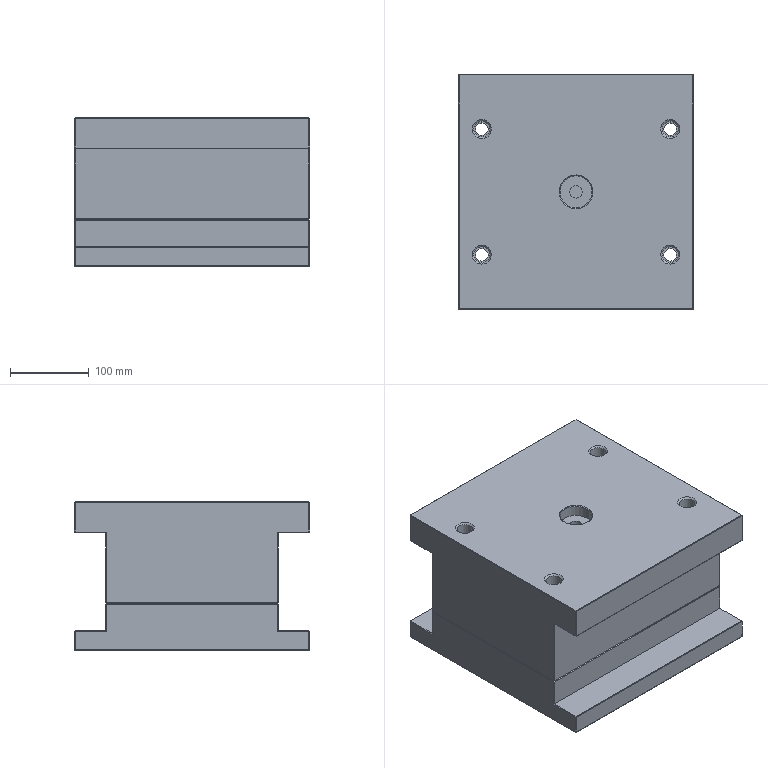NC program | NX | posted with a generic post | part box 300 x 300 x 190 mm
Lines 9219 to 10052 of 34829:
(CAVITY_MILL_COPY_COPY_COPY , TOOL : D6)
N18436 T06 M6
N18438 G17 G43 G0 G90 X-0.783 Y1.63 Z30. S2500 H6 M3
N18440 Z-58.5
N18442 G94 G1 X-1.101 Y1.448 Z-58.519 F1000.
N18444 X-1.436 Y1.116 Z-58.544
N18446 X-1.637 Y0.793 Z-58.564
N18448 X-1.795 Y0.295 Z-58.591
N18450 X-1.805 Y-0.227 Z-58.619
N18452 X-1.666 Y-0.731 Z-58.646
N18454 X-1.389 Y-1.174 Z-58.673
N18456 X-0.999 Y-1.52 Z-58.701
N18458 X-0.526 Y-1.741 Z-58.728
N18460 X-0.151 Y-1.813 Z-58.748
N18462 X0.002 Y-1.819 Z-58.756
N18464 X0.38 Y-1.779 Z-58.776
N18466 X0.81 Y-1.628 Z-58.8
N18468 X1.189 Y-1.376 Z-58.824
N18470 X1.494 Y-1.037 Z-58.848
N18472 X1.705 Y-0.634 Z-58.871
N18474 X1.809 Y-0.19 Z-58.895
N18476 Y0.19 Z-58.915
N18478 X1.749 Y0.499 Z-58.932
N18480 X1.637 Y0.793 Z-58.948
N18482 X1.436 Y1.116 Z-58.968
N18484 X1.101 Y1.448 Z-58.993
N18486 X0.692 Y1.682 Z-59.018
N18488 X0.236 Y1.804 Z-59.042
N18490 X-0.236 Z-59.067
N18492 X-0.692 Y1.682 Z-59.092
N18494 X-1.101 Y1.448 Z-59.117
N18496 X-1.436 Y1.116 Z-59.141
N18498 X-1.637 Y0.793 Z-59.161
N18500 X-1.795 Y0.295 Z-59.189
N18502 X-1.805 Y-0.227 Z-59.216
N18504 X-1.666 Y-0.731 Z-59.243
N18506 X-1.389 Y-1.174 Z-59.271
N18508 X-0.999 Y-1.52 Z-59.298
N18510 X-0.526 Y-1.741 Z-59.325
N18512 X-0.151 Y-1.813 Z-59.345
N18514 X0.002 Y-1.819 Z-59.353
N18516 X0.38 Y-1.779 Z-59.373
N18518 X0.81 Y-1.628 Z-59.397
N18520 X1.189 Y-1.376 Z-59.421
N18522 X1.494 Y-1.037 Z-59.445
N18524 X1.705 Y-0.634 Z-59.469
N18526 X1.809 Y-0.19 Z-59.493
N18528 Y0.19 Z-59.513
N18530 X1.749 Y0.499 Z-59.529
N18532 X1.637 Y0.793 Z-59.546
N18534 X1.436 Y1.116 Z-59.566
N18536 X1.101 Y1.448 Z-59.59
N18538 X0.692 Y1.682 Z-59.615
N18540 X0.236 Y1.804 Z-59.64
N18542 X-0.236 Z-59.664
N18544 X-0.692 Y1.682 Z-59.689
N18546 X-1.101 Y1.448 Z-59.714
N18548 X-1.436 Y1.116 Z-59.739
N18550 X-1.637 Y0.793 Z-59.759
N18552 X-1.795 Y0.295 Z-59.786
N18554 X-1.805 Y-0.227 Z-59.813
N18556 X-1.666 Y-0.731 Z-59.841
N18558 X-1.389 Y-1.174 Z-59.868
N18560 X-0.999 Y-1.52 Z-59.895
N18562 X-0.526 Y-1.741 Z-59.923
N18564 X-0.151 Y-1.813 Z-59.943
N18566 X0.002 Y-1.819 Z-59.951
N18568 X0.38 Y-1.779 Z-59.971
N18570 X0.81 Y-1.628 Z-59.995
N18572 X1.189 Y-1.376 Z-60.018
N18574 X1.494 Y-1.037 Z-60.042
N18576 X1.705 Y-0.634 Z-60.066
N18578 X1.809 Y-0.19 Z-60.09
N18580 Y0. Z-60.1
N18582 G3 X0. Y1.809 R1.809 F1500.
N18584 X1.809 Y0. R-1.809
N18586 G1 X5.709
N18588 G3 X0. Y5.709 R5.709
N18590 X5.709 Y0. R-5.709
N18592 G1 X9.609
N18594 G3 X0. Y9.609 R9.609
N18596 X9.609 Y0. R-9.609
N18598 G1 X13.509
N18600 G3 X0. Y13.509 R13.509
N18602 X13.509 Y0. R-13.509
N18604 G1 X17.409
N18606 G3 X0. Y17.409 R17.409
N18608 X17.409 Y0. R-17.409
N18610 G1 X21.309
N18612 G3 X0. Y21.309 R21.309
N18614 X21.309 Y0. R-21.309
N18616 X20.809 Y0.866 R1.
N18618 G1 Z-58.6
N18620 G0 Z30.
N18622 X-0.063 Y-1.766
N18624 Z-58.6
N18626 G1 X-0.001 Y-1.768 Z-58.603 F1000.
N18628 X0.186 Y-1.748 Z-58.613
N18630 X0.373 Y-1.728 Z-58.623
N18632 X0.802 Y-1.576 Z-58.647
N18634 X1.178 Y-1.318 Z-58.671
N18636 X1.476 Y-0.973 Z-58.695
N18638 X1.676 Y-0.564 Z-58.718
N18640 X1.764 Y-0.117 Z-58.742
N18642 X1.735 Y0.338 Z-58.766
N18644 X1.591 Y0.771 Z-58.79
N18646 X1.393 Y1.089 Z-58.81
N18648 X1.067 Y1.41 Z-58.834
N18650 X0.67 Y1.636 Z-58.858
N18652 X0.228 Y1.753 Z-58.882
N18654 X-0.228 Z-58.906
N18656 X-0.67 Y1.636 Z-58.93
N18658 X-1.067 Y1.41 Z-58.953
N18660 X-1.393 Y1.089 Z-58.977
N18662 X-1.591 Y0.771 Z-58.997
N18664 X-1.7 Y0.486 Z-59.013
N18666 X-1.758 Y0.188 Z-59.029
N18668 Y-0.188 Z-59.049
N18670 X-1.627 Y-0.692 Z-59.076
N18672 X-1.355 Y-1.136 Z-59.103
N18674 X-0.965 Y-1.481 Z-59.131
N18676 X-0.491 Y-1.698 Z-59.158
N18678 X-0.122 Y-1.764 Z-59.178
N18680 X-0.001 Y-1.768 Z-59.184
N18682 X0.186 Y-1.748 Z-59.194
N18684 X0.373 Y-1.728 Z-59.204
N18686 X0.802 Y-1.576 Z-59.227
N18688 X1.178 Y-1.318 Z-59.251
N18690 X1.476 Y-0.973 Z-59.275
N18692 X1.676 Y-0.564 Z-59.299
N18694 X1.764 Y-0.117 Z-59.323
N18696 X1.735 Y0.338 Z-59.347
N18698 X1.591 Y0.771 Z-59.371
N18700 X1.393 Y1.089 Z-59.39
N18702 X1.067 Y1.41 Z-59.414
N18704 X0.67 Y1.636 Z-59.438
N18706 X0.228 Y1.753 Z-59.462
N18708 X-0.228 Z-59.486
N18710 X-0.67 Y1.636 Z-59.51
N18712 X-1.067 Y1.41 Z-59.534
N18714 X-1.393 Y1.089 Z-59.558
N18716 X-1.591 Y0.771 Z-59.578
N18718 X-1.7 Y0.486 Z-59.594
N18720 X-1.758 Y0.188 Z-59.61
N18722 Y-0.188 Z-59.629
N18724 X-1.627 Y-0.692 Z-59.657
N18726 X-1.355 Y-1.136 Z-59.684
N18728 X-0.965 Y-1.481 Z-59.711
N18730 X-0.491 Y-1.698 Z-59.738
N18732 X-0.122 Y-1.764 Z-59.758
N18734 X-0.001 Y-1.768 Z-59.764
N18736 X0.186 Y-1.748 Z-59.774
N18738 X0.373 Y-1.728 Z-59.784
N18740 X0.802 Y-1.576 Z-59.808
N18742 X1.178 Y-1.318 Z-59.832
N18744 X1.476 Y-0.973 Z-59.856
N18746 X1.676 Y-0.564 Z-59.88
N18748 X1.764 Y-0.117 Z-59.904
N18750 X1.735 Y0.338 Z-59.927
N18752 X1.591 Y0.771 Z-59.951
N18754 X1.393 Y1.089 Z-59.971
N18756 X1.067 Y1.41 Z-59.995
N18758 X0.67 Y1.636 Z-60.019
N18760 X0.228 Y1.753 Z-60.043
N18762 X-0.228 Z-60.067
N18764 X-0.67 Y1.636 Z-60.091
N18766 X-1.067 Y1.41 Z-60.115
N18768 X-1.393 Y1.089 Z-60.139
N18770 X-1.591 Y0.771 Z-60.158
N18772 X-1.7 Y0.486 Z-60.174
N18774 X-1.758 Y0.188 Z-60.19
N18776 Y0. Z-60.2
N18778 G3 X0. Y-1.758 R1.758 F1500.
N18780 X-1.758 Y0. R-1.758
N18782 G1 X-5.658
N18784 G3 X0. Y-5.658 R5.658
N18786 X-5.658 Y0. R-5.658
N18788 G1 X-9.558
N18790 G3 X0. Y-9.558 R9.558
N18792 X-9.558 Y0. R-9.558
N18794 G1 X-13.458
N18796 G3 X0. Y-13.458 R13.458
N18798 X-13.458 Y0. R-13.458
N18800 G1 X-17.358
N18802 G3 X0. Y-17.358 R17.358
N18804 X-17.358 Y0. R-17.358
N18806 G1 X-21.258
N18808 G3 X0. Y-21.258 R21.258
N18810 X-21.258 Y0. R-21.258
N18812 X-20.758 Y-0.866 R1.
N18814 G1 Z-58.7
N18816 G0 Z30.
N18818 X-0.913 Y-1.452
N18820 Z-58.7
N18822 G1 X-0.456 Y-1.655 Z-58.726 F1000.
N18824 X-0.274 Y-1.685 Z-58.736
N18826 X-0.091 Y-1.715 Z-58.746
N18828 X-0.003 Y-1.717 Z-58.75
N18830 X0.365 Y-1.678 Z-58.77
N18832 X0.846 Y-1.494 Z-58.797
N18834 X1.251 Y-1.175 Z-58.824
N18836 X1.544 Y-0.751 Z-58.851
N18838 X1.697 Y-0.259 Z-58.878
N18840 X1.698 Y0.256 Z-58.905
N18842 X1.545 Y0.748 Z-58.932
N18844 X1.349 Y1.062 Z-58.951
N18846 X0.973 Y1.415 Z-58.978
N18848 X0.51 Y1.64 Z-59.005
N18850 X0. Y1.717 Z-59.032
N18852 X-0.51 Y1.64 Z-59.059
N18854 X-0.973 Y1.415 Z-59.086
N18856 X-1.349 Y1.062 Z-59.113
N18858 X-1.545 Y0.748 Z-59.132
N18860 X-1.65 Y0.474 Z-59.148
N18862 X-1.707 Y0.185 Z-59.163
N18864 Y-0.185 Z-59.183
N18866 X-1.577 Y-0.679 Z-59.209
N18868 X-1.308 Y-1.112 Z-59.236
N18870 X-0.923 Y-1.448 Z-59.263
N18872 X-0.456 Y-1.655 Z-59.29
N18874 X-0.274 Y-1.685 Z-59.299
N18876 X-0.091 Y-1.715 Z-59.309
N18878 X-0.003 Y-1.717 Z-59.314
N18880 X0.365 Y-1.678 Z-59.333
N18882 X0.846 Y-1.494 Z-59.36
N18884 X1.251 Y-1.175 Z-59.387
N18886 X1.544 Y-0.751 Z-59.414
N18888 X1.697 Y-0.259 Z-59.441
N18890 X1.698 Y0.256 Z-59.468
N18892 X1.545 Y0.748 Z-59.495
N18894 X1.349 Y1.062 Z-59.515
N18896 X0.973 Y1.415 Z-59.542
N18898 X0.51 Y1.64 Z-59.569
N18900 X0. Y1.717 Z-59.596
N18902 X-0.51 Y1.64 Z-59.623
N18904 X-0.973 Y1.415 Z-59.65
N18906 X-1.349 Y1.062 Z-59.677
N18908 X-1.545 Y0.748 Z-59.696
N18910 X-1.65 Y0.474 Z-59.711
N18912 X-1.707 Y0.185 Z-59.727
N18914 Y-0.185 Z-59.746
N18916 X-1.577 Y-0.679 Z-59.773
N18918 X-1.308 Y-1.112 Z-59.8
N18920 X-0.923 Y-1.448 Z-59.826
N18922 X-0.456 Y-1.655 Z-59.853
N18924 X-0.274 Y-1.685 Z-59.863
N18926 X-0.091 Y-1.715 Z-59.873
N18928 X-0.003 Y-1.717 Z-59.877
N18930 X0.365 Y-1.678 Z-59.897
N18932 X0.846 Y-1.494 Z-59.924
N18934 X1.251 Y-1.175 Z-59.951
N18936 X1.544 Y-0.751 Z-59.978
N18938 X1.697 Y-0.259 Z-60.005
N18940 X1.698 Y0.256 Z-60.032
N18942 X1.545 Y0.748 Z-60.059
N18944 X1.349 Y1.062 Z-60.078
N18946 X0.973 Y1.415 Z-60.105
N18948 X0.51 Y1.64 Z-60.132
N18950 X0. Y1.717 Z-60.159
N18952 X-0.51 Y1.64 Z-60.186
N18954 X-0.973 Y1.415 Z-60.213
N18956 X-1.349 Y1.062 Z-60.24
N18958 X-1.545 Y0.748 Z-60.259
N18960 X-1.65 Y0.474 Z-60.275
N18962 X-1.707 Y0.185 Z-60.29
N18964 Y0. Z-60.3
N18966 G3 X0. Y-1.707 R1.707 F1500.
N18968 X-1.707 Y0. R-1.707
N18970 G1 X-5.607
N18972 G3 X0. Y-5.607 R5.607
N18974 X-5.607 Y0. R-5.607
N18976 G1 X-9.507
N18978 G3 X0. Y-9.507 R9.507
N18980 X-9.507 Y0. R-9.507
N18982 G1 X-13.407
N18984 G3 X0. Y-13.407 R13.407
N18986 X-13.407 Y0. R-13.407
N18988 G1 X-17.307
N18990 G3 X0. Y-17.307 R17.307
N18992 X-17.307 Y0. R-17.307
N18994 G1 X-21.207
N18996 G3 X0. Y-21.207 R21.207
N18998 X-21.207 Y0. R-21.207
N19000 X-20.707 Y-0.866 R1.
N19002 G1 Z-58.8
N19004 G0 Z30.
N19006 X-0.742 Y1.477
N19008 Z-58.8
N19010 G1 X-0.991 Y1.339 Z-58.815 F1000.
N19012 X-1.306 Y1.035 Z-58.838
N19014 X-1.5 Y0.726 Z-58.857
N19016 X-1.646 Y0.259 Z-58.883
N19018 X-1.65 Y-0.229 Z-58.908
N19020 X-1.513 Y-0.698 Z-58.934
N19022 X-1.245 Y-1.107 Z-58.959
N19024 X-0.87 Y-1.421 Z-58.985
N19026 X-0.421 Y-1.612 Z-59.011
N19028 X-0.24 Y-1.638 Z-59.02
N19030 X-0.06 Y-1.665 Z-59.03
N19032 X-0.005 Y-1.666 Z-59.033
N19034 X0.357 Y-1.627 Z-59.052
N19036 X0.824 Y-1.448 Z-59.078
N19038 X1.216 Y-1.139 Z-59.104
N19040 X1.499 Y-0.728 Z-59.13
N19042 X1.647 Y-0.251 Z-59.156
N19044 Y0.249 Z-59.183
N19046 X1.5 Y0.726 Z-59.209
N19048 X1.306 Y1.035 Z-59.228
N19050 X0.991 Y1.339 Z-59.251
N19052 X0.608 Y1.551 Z-59.274
N19054 X0.182 Y1.656 Z-59.297
N19056 X-0.182 Z-59.316
N19058 X-0.608 Y1.551 Z-59.339
N19060 X-0.991 Y1.339 Z-59.362
N19062 X-1.306 Y1.035 Z-59.385
N19064 X-1.5 Y0.726 Z-59.404
N19066 X-1.646 Y0.259 Z-59.429
N19068 X-1.65 Y-0.229 Z-59.455
N19070 X-1.513 Y-0.698 Z-59.481
N19072 X-1.245 Y-1.107 Z-59.506
N19074 X-0.87 Y-1.421 Z-59.532
N19076 X-0.421 Y-1.612 Z-59.558
N19078 X-0.24 Y-1.638 Z-59.567
N19080 X-0.06 Y-1.665 Z-59.577
N19082 X-0.005 Y-1.666 Z-59.579
N19084 X0.357 Y-1.627 Z-59.599
N19086 X0.824 Y-1.448 Z-59.625
N19088 X1.216 Y-1.139 Z-59.651
N19090 X1.499 Y-0.728 Z-59.677
N19092 X1.647 Y-0.251 Z-59.703
N19094 Y0.249 Z-59.729
N19096 X1.5 Y0.726 Z-59.756
N19098 X1.306 Y1.035 Z-59.775
N19100 X0.991 Y1.339 Z-59.798
N19102 X0.608 Y1.551 Z-59.821
N19104 X0.182 Y1.656 Z-59.844
N19106 X-0.182 Z-59.863
N19108 X-0.608 Y1.551 Z-59.886
N19110 X-0.991 Y1.339 Z-59.909
N19112 X-1.306 Y1.035 Z-59.932
N19114 X-1.5 Y0.726 Z-59.951
N19116 X-1.646 Y0.259 Z-59.976
N19118 X-1.65 Y-0.229 Z-60.002
N19120 X-1.513 Y-0.698 Z-60.028
N19122 X-1.245 Y-1.107 Z-60.053
N19124 X-0.87 Y-1.421 Z-60.079
N19126 X-0.421 Y-1.612 Z-60.104
N19128 X-0.24 Y-1.638 Z-60.114
N19130 X-0.06 Y-1.665 Z-60.123
N19132 X-0.005 Y-1.666 Z-60.126
N19134 X0.357 Y-1.627 Z-60.145
N19136 X0.824 Y-1.448 Z-60.172
N19138 X1.216 Y-1.139 Z-60.198
N19140 X1.499 Y-0.728 Z-60.224
N19142 X1.647 Y-0.251 Z-60.25
N19144 Y0.249 Z-60.276
N19146 X1.5 Y0.726 Z-60.302
N19148 X1.306 Y1.035 Z-60.322
N19150 X0.991 Y1.339 Z-60.345
N19152 X0.608 Y1.551 Z-60.367
N19154 X0.182 Y1.656 Z-60.39
N19156 X0. Z-60.4
N19158 G3 X-1.656 Y0. R1.656 F1500.
N19160 X0. Y1.656 R-1.656
N19162 G1 Y5.556
N19164 G3 X-5.556 Y0. R5.556
N19166 X0. Y5.556 R-5.556
N19168 G1 Y9.456
N19170 G3 X-9.456 Y0. R9.456
N19172 X0. Y9.456 R-9.456
N19174 G1 Y13.356
N19176 G3 X-13.356 Y0. R13.356
N19178 X0. Y13.356 R-13.356
N19180 G1 Y17.256
N19182 G3 X-17.256 Y0. R17.256
N19184 X0. Y17.256 R-17.256
N19186 G1 Y21.156
N19188 G3 X-21.156 Y0. R21.156
N19190 X0. Y21.156 R-21.156
N19192 X-0.866 Y20.656 R1.
N19194 G1 Z-58.9
N19196 G0 Z30.
N19198 X1.603 Y-0.188
N19200 Z-58.9
N19202 G1 X1.605 Y-0.179 F1000.
N19204 Y0.179 Z-58.919
N19206 X1.552 Y0.448 Z-58.934
N19208 X1.454 Y0.703 Z-58.948
N19210 X1.263 Y1.007 Z-58.967
N19212 X0.91 Y1.334 Z-58.992
N19214 X0.476 Y1.543 Z-59.017
N19216 X0. Y1.615 Z-59.042
N19218 X-0.476 Y1.543 Z-59.068
N19220 X-0.91 Y1.334 Z-59.093
N19222 X-1.263 Y1.007 Z-59.118
N19224 X-1.454 Y0.703 Z-59.137
N19226 X-1.596 Y0.247 Z-59.162
N19228 X-1.598 Y-0.231 Z-59.187
N19230 X-1.461 Y-0.689 Z-59.212
N19232 X-1.195 Y-1.086 Z-59.237
N19234 X-0.825 Y-1.388 Z-59.262
N19236 X-0.383 Y-1.569 Z-59.287
N19238 X-0.027 Y-1.615 Z-59.306
N19240 X-0.007 Z-59.307
N19242 X0.349 Y-1.577 Z-59.326
N19244 X0.814 Y-1.395 Z-59.352
N19246 X1.201 Y-1.079 Z-59.378
N19248 X1.474 Y-0.661 Z-59.404
N19250 X1.605 Y-0.179 Z-59.431
N19252 Y0.179 Z-59.449
N19254 X1.552 Y0.448 Z-59.464
N19256 X1.454 Y0.703 Z-59.478
N19258 X1.263 Y1.007 Z-59.497
N19260 X0.91 Y1.334 Z-59.522
N19262 X0.476 Y1.543 Z-59.547
N19264 X0. Y1.615 Z-59.572
N19266 X-0.476 Y1.543 Z-59.598
N19268 X-0.91 Y1.334 Z-59.623
N19270 X-1.263 Y1.007 Z-59.648
N19272 X-1.454 Y0.703 Z-59.667
N19274 X-1.596 Y0.247 Z-59.692
N19276 X-1.598 Y-0.231 Z-59.717
N19278 X-1.461 Y-0.689 Z-59.742
N19280 X-1.195 Y-1.086 Z-59.767
N19282 X-0.825 Y-1.388 Z-59.792
N19284 X-0.383 Y-1.569 Z-59.817
N19286 X-0.027 Y-1.615 Z-59.836
N19288 X-0.007 Z-59.837
N19290 X0.349 Y-1.577 Z-59.856
N19292 X0.814 Y-1.395 Z-59.882
N19294 X1.201 Y-1.079 Z-59.908
N19296 X1.474 Y-0.661 Z-59.934
N19298 X1.605 Y-0.179 Z-59.961
N19300 Y0.179 Z-59.979
N19302 X1.552 Y0.448 Z-59.994
N19304 X1.454 Y0.703 Z-60.008
N19306 X1.263 Y1.007 Z-60.027
N19308 X0.91 Y1.334 Z-60.052
N19310 X0.476 Y1.543 Z-60.077
N19312 X0. Y1.615 Z-60.103
N19314 X-0.476 Y1.543 Z-60.128
N19316 X-0.91 Y1.334 Z-60.153
N19318 X-1.263 Y1.007 Z-60.178
N19320 X-1.454 Y0.703 Z-60.197
N19322 X-1.596 Y0.247 Z-60.222
N19324 X-1.598 Y-0.231 Z-60.247
N19326 X-1.461 Y-0.689 Z-60.272
N19328 X-1.195 Y-1.086 Z-60.297
N19330 X-0.825 Y-1.388 Z-60.322
N19332 X-0.383 Y-1.569 Z-60.347
N19334 X-0.027 Y-1.615 Z-60.366
N19336 X-0.007 Z-60.367
N19338 X0.349 Y-1.577 Z-60.386
N19340 X0.814 Y-1.395 Z-60.412
N19342 X1.201 Y-1.079 Z-60.438
N19344 X1.474 Y-0.661 Z-60.464
N19346 X1.605 Y-0.179 Z-60.491
N19348 Y0. Z-60.5
N19350 G3 X0. Y1.605 R1.605 F1500.
N19352 X1.605 Y0. R-1.605
N19354 G1 X5.505
N19356 G3 X0. Y5.505 R5.505
N19358 X5.505 Y0. R-5.505
N19360 G1 X9.405
N19362 G3 X0. Y9.405 R9.405
N19364 X9.405 Y0. R-9.405
N19366 G1 X13.305
N19368 G3 X0. Y13.305 R13.305
N19370 X13.305 Y0. R-13.305
N19372 G1 X17.205
N19374 G3 X0. Y17.205 R17.205
N19376 X17.205 Y0. R-17.205
N19378 G1 X21.105
N19380 G3 X0. Y21.105 R21.105
N19382 X21.105 Y0. R-21.105
N19384 X20.605 Y0.866 R1.
N19386 G1 Z-59.
N19388 G0 Z30.
N19390 X1.159 Y-1.049
N19392 Z-59.
N19394 G1 X1.164 Y-1.045 F1000.
N19396 X1.427 Y-0.641 Z-59.026
N19398 X1.554 Y-0.177 Z-59.051
N19400 Y0.177 Z-59.069
N19402 X1.502 Y0.435 Z-59.083
N19404 X1.408 Y0.681 Z-59.097
N19406 X1.22 Y0.979 Z-59.115
N19408 X0.878 Y1.295 Z-59.14
N19410 X0.459 Y1.495 Z-59.164
N19412 X-0.001 Y1.564 Z-59.189
N19414 X-0.461 Y1.495 Z-59.213
N19416 X-0.88 Y1.293 Z-59.237
N19418 X-1.221 Y0.977 Z-59.262
N19420 X-1.409 Y0.678 Z-59.28
N19422 X-1.547 Y0.232 Z-59.305
N19424 X-1.546 Y-0.235 Z-59.329
N19426 X-1.408 Y-0.681 Z-59.354
N19428 X-1.144 Y-1.067 Z-59.378
N19430 X-0.778 Y-1.357 Z-59.403
N19432 X-0.342 Y-1.526 Z-59.427
N19434 X0. Y-1.563 Z-59.445
N19436 X0.342 Y-1.526 Z-59.463
N19438 X0.79 Y-1.35 Z-59.488
N19440 X1.164 Y-1.045 Z-59.514
N19442 X1.427 Y-0.641 Z-59.539
N19444 X1.554 Y-0.177 Z-59.564
N19446 Y0.177 Z-59.583
N19448 X1.502 Y0.435 Z-59.596
N19450 X1.408 Y0.681 Z-59.61
N19452 X1.22 Y0.979 Z-59.629
N19454 X0.878 Y1.295 Z-59.653
N19456 X0.459 Y1.495 Z-59.677
N19458 X-0.001 Y1.564 Z-59.702
N19460 X-0.461 Y1.495 Z-59.726
N19462 X-0.88 Y1.293 Z-59.751
N19464 X-1.221 Y0.977 Z-59.775
N19466 X-1.409 Y0.678 Z-59.793
N19468 X-1.547 Y0.232 Z-59.818
N19470 X-1.546 Y-0.235 Z-59.842
N19472 X-1.408 Y-0.681 Z-59.867
N19474 X-1.144 Y-1.067 Z-59.891
N19476 X-0.778 Y-1.357 Z-59.916
N19478 X-0.342 Y-1.526 Z-59.94
N19480 X0. Y-1.563 Z-59.958
N19482 X0.342 Y-1.526 Z-59.976
N19484 X0.79 Y-1.35 Z-60.002
N19486 X1.164 Y-1.045 Z-60.027
N19488 X1.427 Y-0.641 Z-60.052
N19490 X1.554 Y-0.177 Z-60.077
N19492 Y0.177 Z-60.096
N19494 X1.502 Y0.435 Z-60.11
N19496 X1.408 Y0.681 Z-60.124
N19498 X1.22 Y0.979 Z-60.142
N19500 X0.878 Y1.295 Z-60.166
N19502 X0.459 Y1.495 Z-60.191
N19504 X-0.001 Y1.564 Z-60.215
N19506 X-0.461 Y1.495 Z-60.24
N19508 X-0.88 Y1.293 Z-60.264
N19510 X-1.221 Y0.977 Z-60.288
N19512 X-1.409 Y0.678 Z-60.307
N19514 X-1.547 Y0.232 Z-60.331
N19516 X-1.546 Y-0.235 Z-60.356
N19518 X-1.408 Y-0.681 Z-60.38
N19520 X-1.144 Y-1.067 Z-60.405
N19522 X-0.778 Y-1.357 Z-60.429
N19524 X-0.342 Y-1.526 Z-60.454
N19526 X0. Y-1.563 Z-60.472
N19528 X0.342 Y-1.526 Z-60.49
N19530 X0.79 Y-1.35 Z-60.515
N19532 X1.164 Y-1.045 Z-60.54
N19534 X1.427 Y-0.641 Z-60.565
N19536 X1.554 Y-0.177 Z-60.591
N19538 Y0. Z-60.6
N19540 G3 X0. Y1.554 R1.554 F1500.
N19542 X1.554 Y0. R-1.554
N19544 G1 X5.454
N19546 G3 X0. Y5.454 R5.454
N19548 X5.454 Y0. R-5.454
N19550 G1 X9.354
N19552 G3 X0. Y9.354 R9.354
N19554 X9.354 Y0. R-9.354
N19556 G1 X13.254
N19558 G3 X0. Y13.254 R13.254
N19560 X13.254 Y0. R-13.254
N19562 G1 X17.154
N19564 G3 X0. Y17.154 R17.154
N19566 X17.154 Y0. R-17.154
N19568 G1 X21.054
N19570 G3 X0. Y21.054 R21.054
N19572 X21.054 Y0. R-21.054
N19574 X20.554 Y0.866 R1.
N19576 G1 Z-59.1
N19578 G0 Z30.
N19580 X-0.268 Y1.473
N19582 Z-59.1
N19584 G1 X-0.433 Y1.45 Z-59.109 F1000.
N19586 X-0.843 Y1.257 Z-59.132
N19588 X-1.177 Y0.951 Z-59.156
N19590 X-1.363 Y0.658 Z-59.174
N19592 X-1.453 Y0.422 Z-59.188
N19594 X-1.503 Y0.174 Z-59.201
N19596 Y-0.174 Z-59.219
N19598 X-1.394 Y-0.59 Z-59.242
N19600 X-1.171 Y-0.958 Z-59.264
N19602 X-0.854 Y-1.249 Z-59.287
N19604 X-0.468 Y-1.439 Z-59.309
N19606 X-0.128 Y-1.508 Z-59.328
N19608 X-0.037 Y-1.513 Z-59.332
N19610 X0.136 Y-1.497 Z-59.341
N19612 X0.309 Y-1.481 Z-59.351
N19614 X0.732 Y-1.324 Z-59.374
N19616 X1.09 Y-1.05 Z-59.398
N19618 X1.351 Y-0.682 Z-59.421
N19620 X1.492 Y-0.253 Z-59.445
N19622 X1.5 Y0.198 Z-59.469
N19624 X1.375 Y0.632 Z-59.492
N19626 X1.195 Y0.928 Z-59.511
N19628 X0.867 Y1.24 Z-59.534
N19630 X0.461 Y1.441 Z-59.558
N19632 X0.015 Y1.513 Z-59.582
N19634 X-0.433 Y1.45 Z-59.605
N19636 X-0.843 Y1.257 Z-59.629
N19638 X-1.177 Y0.951 Z-59.653
N19640 X-1.363 Y0.658 Z-59.671
N19642 X-1.453 Y0.422 Z-59.684
N19644 X-1.503 Y0.174 Z-59.698
N19646 Y-0.174 Z-59.716
N19648 X-1.394 Y-0.59 Z-59.738
N19650 X-1.171 Y-0.958 Z-59.761
N19652 X-0.854 Y-1.249 Z-59.783
N19654 X-0.468 Y-1.439 Z-59.806
N19656 X-0.128 Y-1.508 Z-59.824
N19658 X-0.037 Y-1.513 Z-59.829
N19660 X0.136 Y-1.497 Z-59.838
N19662 X0.309 Y-1.481 Z-59.847
N19664 X0.732 Y-1.324 Z-59.871
N19666 X1.09 Y-1.05 Z-59.894
N19668 X1.351 Y-0.682 Z-59.918
N19670 X1.492 Y-0.253 Z-59.942
N19672 X1.5 Y0.198 Z-59.965
N19674 X1.375 Y0.632 Z-59.989
N19676 X1.195 Y0.928 Z-60.007
N19678 X0.867 Y1.24 Z-60.031
N19680 X0.461 Y1.441 Z-60.055
N19682 X0.015 Y1.513 Z-60.078
N19684 X-0.433 Y1.45 Z-60.102
N19686 X-0.843 Y1.257 Z-60.126
N19688 X-1.177 Y0.951 Z-60.15
N19690 X-1.363 Y0.658 Z-60.168
N19692 X-1.453 Y0.422 Z-60.181
N19694 X-1.503 Y0.174 Z-60.194
N19696 Y-0.174 Z-60.212
N19698 X-1.394 Y-0.59 Z-60.235
N19700 X-1.171 Y-0.958 Z-60.258
N19702 X-0.854 Y-1.249 Z-60.28
N19704 X-0.468 Y-1.439 Z-60.303
N19706 X-0.128 Y-1.508 Z-60.321
N19708 X-0.037 Y-1.513 Z-60.326
N19710 X0.136 Y-1.497 Z-60.335
N19712 X0.309 Y-1.481 Z-60.344
N19714 X0.732 Y-1.324 Z-60.367
N19716 X1.09 Y-1.05 Z-60.391
N19718 X1.351 Y-0.682 Z-60.415
N19720 X1.492 Y-0.253 Z-60.438
N19722 X1.5 Y0.198 Z-60.462
N19724 X1.375 Y0.632 Z-60.486
N19726 X1.195 Y0.928 Z-60.504
N19728 X0.867 Y1.24 Z-60.528
N19730 X0.461 Y1.441 Z-60.551
N19732 X0.015 Y1.513 Z-60.575
N19734 X-0.433 Y1.45 Z-60.599
N19736 X-0.843 Y1.257 Z-60.622
N19738 X-1.177 Y0.951 Z-60.646
N19740 X-1.363 Y0.658 Z-60.664
N19742 X-1.453 Y0.422 Z-60.678
N19744 X-1.503 Y0.174 Z-60.691
N19746 Y0. Z-60.7
N19748 G3 X0. Y-1.503 R1.503 F1500.
N19750 X-1.503 Y0. R-1.503
N19752 G1 X-5.403
N19754 G3 X0. Y-5.403 R5.403
N19756 X-5.403 Y0. R-5.403
N19758 G1 X-9.303
N19760 G3 X0. Y-9.303 R9.303
N19762 X-9.303 Y0. R-9.303
N19764 G1 X-13.203
N19766 G3 X0. Y-13.203 R13.203
N19768 X-13.203 Y0. R-13.203
N19770 G1 X-17.103
N19772 G3 X0. Y-17.103 R17.103
N19774 X-17.103 Y0. R-17.103
N19776 G1 X-21.003
N19778 G3 X0. Y-21.003 R21.003
N19780 X-21.003 Y0. R-21.003
N19782 X-20.503 Y-0.866 R1.
N19784 G1 Z-59.2
N19786 G0 Z30.
N19788 X-2.948 Y4.462
N19790 Z-59.2
N19792 G1 X-3.242 Y4.271 Z-59.218 F1000.
N19794 X-3.832 Y3.75 Z-59.26
N19796 X-4.34 Y3.149 Z-59.301
N19798 X-4.692 Y2.596 Z-59.335
N19800 X-5.057 Y1.784 Z-59.382
N19802 X-5.282 Y0.923 Z-59.428
N19804 X-5.362 Y0.037 Z-59.475
N19806 X-5.294 Y-0.851 Z-59.522
N19808 X-5.081 Y-1.715 Z-59.568
N19810 X-4.727 Y-2.532 Z-59.615
N19812 X-4.243 Y-3.279 Z-59.662
N19814 X-3.642 Y-3.935 Z-59.708
N19816 X-2.941 Y-4.484 Z-59.755
N19818 X-2.159 Y-4.908 Z-59.802
N19820 X-1.317 Y-5.198 Z-59.848
N19822 X-0.674 Y-5.32 Z-59.883
N19824 X0.16 Y-5.36 Z-59.926
N19826 X0.812 Y-5.3 Z-59.961
N19828 X1.64 Y-5.105 Z-60.005
N19830 X2.426 Y-4.782 Z-60.05
N19832 X3.151 Y-4.338 Z-60.094
N19834 X3.797 Y-3.786 Z-60.139
N19836 X4.348 Y-3.138 Z-60.183
N19838 X4.789 Y-2.411 Z-60.228
N19840 X5.11 Y-1.624 Z-60.273
N19842 X5.303 Y-0.796 Z-60.317
N19844 X5.362 Y0.052 Z-60.362
N19846 X5.286 Y0.899 Z-60.406
N19848 X5.078 Y1.724 Z-60.451
N19850 X4.741 Y2.504 Z-60.495
N19852 X4.401 Y3.064 Z-60.53
N19854 X3.893 Y3.688 Z-60.572
N19856 X3.297 Y4.229 Z-60.614
N19858 X2.626 Y4.675 Z-60.656
N19860 X1.897 Y5.015 Z-60.698
N19862 X1.125 Y5.243 Z-60.741
N19864 X0.327 Y5.352 Z-60.783
N19866 X0. Z-60.8
N19868 Y1.452
N19870 G3 X-1.452 Y0. R1.452 F1500.
N19872 X0. Y1.452 R-1.452
N19874 G1 Y5.352
N19876 G3 X-5.352 Y0. R5.352
N19878 X0. Y5.352 R-5.352
N19880 G1 Y9.252
N19882 G3 X-9.252 Y0. R9.252
N19884 X0. Y9.252 R-9.252
N19886 G1 Y13.152
N19888 G3 X-13.152 Y0. R13.152
N19890 X0. Y13.152 R-13.152
N19892 G1 Y17.052
N19894 G3 X-17.052 Y0. R17.052
N19896 X0. Y17.052 R-17.052
N19898 G1 Y20.952
N19900 G3 X-20.952 Y0. R20.952
N19902 X0. Y20.952 R-20.952
N19904 X-0.866 Y20.452 R1.
N19906 G1 Z-59.3
N19908 G0 Z30.
N19910 X-2.675 Y4.578
N19912 Z-59.3
N19914 G1 X-3.206 Y4.234 Z-59.333 F1000.
N19916 X-3.79 Y3.721 Z-59.374
N19918 X-4.293 Y3.127 Z-59.415
N19920 X-4.644 Y2.577 Z-59.449
N19922 X-5.009 Y1.767 Z-59.495
N19924 X-5.233 Y0.908 Z-59.542
N19926 X-5.311 Y0.022 Z-59.589
N19928 X-5.241 Y-0.863 Z-59.635
N19930 X-5.023 Y-1.725 Z-59.682
N19932 X-4.666 Y-2.538 Z-59.728
N19934 X-4.177 Y-3.28 Z-59.775
N19936 X-3.572 Y-3.931 Z-59.821
N19938 X-2.867 Y-4.471 Z-59.868
N19940 X-2.081 Y-4.887 Z-59.915
N19942 X-1.237 Y-5.165 Z-59.961
N19944 X-0.596 Y-5.278 Z-59.995
N19946 X0.158 Y-5.309 Z-60.035
N19948 X0.807 Y-5.25 Z-60.069
N19950 X1.7 Y-5.032 Z-60.117
N19952 X2.542 Y-4.664 Z-60.165
N19954 X3.307 Y-4.156 Z-60.213
N19956 X3.974 Y-3.524 Z-60.262
N19958 X4.522 Y-2.786 Z-60.31
N19960 X4.934 Y-1.965 Z-60.358
N19962 X5.199 Y-1.085 Z-60.406
N19964 X5.308 Y-0.173 Z-60.454
N19966 X5.259 Y0.745 Z-60.502
N19968 X5.052 Y1.64 Z-60.55
N19970 X4.693 Y2.486 Z-60.599
N19972 X4.354 Y3.042 Z-60.633
N19974 X3.85 Y3.658 Z-60.674
N19976 X3.261 Y4.192 Z-60.716
N19978 X2.598 Y4.632 Z-60.758
N19980 X1.877 Y4.969 Z-60.8
N19982 X1.114 Y5.193 Z-60.841
N19984 X0.326 Y5.301 Z-60.883
N19986 X0. Z-60.9
N19988 Y1.401
N19990 G3 X-1.401 Y0. R1.401 F1500.
N19992 X0. Y1.401 R-1.401
N19994 G1 Y5.301
N19996 G3 X-5.301 Y0. R5.301
N19998 X0. Y5.301 R-5.301
N20000 G1 Y9.201
N20002 G3 X-9.201 Y0. R9.201
N20004 X0. Y9.201 R-9.201
N20006 G1 Y13.101
N20008 G3 X-13.101 Y0. R13.101
N20010 X0. Y13.101 R-13.101
N20012 G1 Y17.001
N20014 G3 X-17.001 Y0. R17.001
N20016 X0. Y17.001 R-17.001
N20018 G1 Y20.901
N20020 G3 X-20.901 Y0. R20.901
N20022 X0. Y20.901 R-20.901
N20024 X-0.866 Y20.401 R1.
N20026 G1 Z-59.4
N20028 G0 Z30.
N20030 X-4.668 Y-2.388
N20032 Z-59.4
N20034 G1 X-4.499 Y-2.726 Z-59.42 F1000.
N20036 X-4.004 Y-3.412 Z-59.464
N20038 X-3.405 Y-4.01 Z-59.508
N20040 X-2.718 Y-4.504 Z-59.553
N20042 X-1.961 Y-4.881 Z-59.597
N20044 X-1.153 Y-5.132 Z-59.642
N20046 X-0.513 Y-5.235 Z-59.676
N20048 X0.156 Y-5.258 Z-59.711
N20050 X0.802 Y-5.199 Z-59.745
N20052 X1.686 Y-4.983 Z-59.792
N20054 X2.52 Y-4.617 Z-59.84
N20056 X3.279 Y-4.114 Z-59.888
N20058 X3.939 Y-3.487 Z-59.935
N20060 X4.481 Y-2.755 Z-59.983
N20062 X4.889 Y-1.942 Z-60.031
N20064 X5.15 Y-1.07 Z-60.079
N20066 X5.258 Y-0.166 Z-60.126
N20068 X5.207 Y0.743 Z-60.174
N20070 X5.001 Y1.63 Z-60.222
N20072 X4.645 Y2.468 Z-60.269
N20074 X4.306 Y3.021 Z-60.303
N20076 X3.724 Y3.716 Z-60.351
N20078 X3.03 Y4.3 Z-60.398
N20080 X2.247 Y4.756 Z-60.446
N20082 X1.396 Y5.072 Z-60.493
N20084 X0.505 Y5.236 Z-60.541
N20086 X-0.402 Y5.245 Z-60.588
N20088 X-1.297 Y5.098 Z-60.636
N20090 X-2.153 Y4.799 Z-60.684
N20092 X-2.945 Y4.358 Z-60.731
N20094 X-3.65 Y3.788 Z-60.779
N20096 X-4.246 Y3.105 Z-60.826